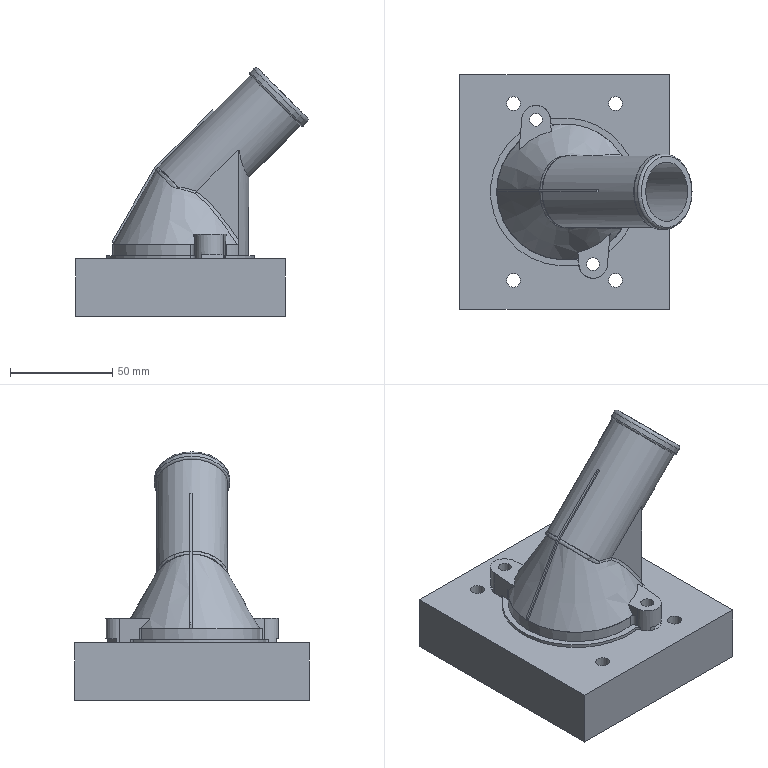NC program | NX | posted by the shop | part box 113.679 x 114.654 x 121.568 mm
Lines 15667 to 16486 of 160120:
15666 TOOL CALL 12 Z S7000
15667 CALL LBL101
15668 M3 M8
15669 M51
15670 CYCL DEF 32.0 TOLERANCE
15671 CYCL DEF 32.1 T0.012
15672 CYCL DEF 32.2 HSC-MODE:0
15673 L M126
15674 L A+0.0 C+0.0 FMAX
15675 L X31.8609 Y9.1209 FMAX
15676 L Z160.5681 FMAX
15677 L Z96.0728 FMAX
15678 L Z95.0728 F1500.
15679 CC X32.458 Y9.9231
15680 C X33.2602 Y9.326 DR+
15681 CC X46.9163 Y-.8392
15682 C X33.3788 Y9.4834 DR- F3000.
15683 CC X62.7458 Y-2.3059
15684 C X33.4604 Y9.6847 DR-
15685 L X33.5103 Y9.8057 Z95.0274
15686 L X33.5614 Y9.9262 Z94.982
15687 L X33.6113 Y10.0472 Z94.9366
15688 L X33.6604 Y10.1685 Z94.8912
15689 L X33.7117 Y10.2889 Z94.8457
15690 L X33.764 Y10.4089 Z94.8003
15691 L X33.8165 Y10.5288 Z94.7549
15692 L X33.8694 Y10.6485 Z94.7095
15693 L X33.9243 Y10.7673 Z94.6641
15694 L X33.979 Y10.8861 Z94.6187
15695 L X34.0305 Y11.0064 Z94.5732
15696 CC X54.2056 Y1.4317
15697 C X33.9017 Y10.7302 DR+
15698 CC X47.0664 Y-1.1912
15699 C X33.6839 Y10.4852 DR+
15700 L X33.7449 Y10.6101 Z94.5177
15701 L X33.8017 Y10.7386 Z94.4622
15702 L X33.8589 Y10.867 Z94.4067
15703 L X33.9187 Y10.9929 Z94.3512
15704 L X33.9813 Y11.1163 Z94.2957
15705 L X34.0439 Y11.2396 Z94.2402
15706 L X34.1065 Y11.3629 Z94.1847
15707 L X34.1699 Y11.4853 Z94.1292
15708 L X34.2302 Y11.6108 Z94.0737
15709 CC X47.4065 Y-1.7424
15710 C X34.4283 Y11.8034 DR-
15711 CC X52.6802 Y2.3208
15712 C X34.5852 Y12.0995 DR-
15713 L X34.6519 Y12.2225 Z94.0112
15714 L X34.72 Y12.3449 Z93.9488
15715 L X34.7889 Y12.4668 Z93.8863
15716 L X34.858 Y12.5886 Z93.8239
15717 L X34.9284 Y12.7096 Z93.7614
15718 L X34.9995 Y12.8303 Z93.699
15719 L X35.0713 Y12.9504 Z93.6365
15720 L X35.1434 Y13.0704 Z93.5741
15721 CC X51.7759 Y2.8978
15722 C X34.9264 Y12.7068 DR+
15723 CC X47.595 Y-2.3086
15724 C X34.6428 Y12.4629 DR+
15725 L X34.7064 Y12.5776 Z93.5027
15726 L X34.7697 Y12.6926 Z93.4314
15727 L X34.8338 Y12.8068 Z93.36
15728 L X34.898 Y12.9207 Z93.2886
15729 L X34.9625 Y13.0344 Z93.2173
15730 L X35.0272 Y13.1477 Z93.1459
15731 L X35.0935 Y13.259 Z93.0745
15732 CC X47.9658 Y-3.0564
15733 C X35.4178 Y13.5097 DR-
15734 CC X51.5003 Y3.067
15735 C X35.6579 Y13.8705 DR-
15736 L X35.7323 Y13.9762 Z93.0031
15737 L X35.8061 Y14.0823 Z92.9318
15738 L X35.8796 Y14.1887 Z92.8604
15739 L X35.9552 Y14.2937 Z92.789
15740 L X36.0312 Y14.3983 Z92.7177
15741 L X36.1073 Y14.5028 Z92.6463
15742 L X36.1847 Y14.6064 Z92.5749
15743 CC X50.2088 Y4.096
15744 C X35.9705 Y14.3144 DR+
15745 CC X35.5058 Y14.6479
15746 C X35.8306 Y14.1771 DR-
15747 CC X48.6089 Y-4.348
15748 C X35.5356 Y13.9701 DR+
15749 L X35.6164 Y14.0815 Z92.4917
15750 L X35.696 Y14.1946 Z92.4084
15751 L X35.773 Y14.3116 Z92.3252
15752 L X35.8559 Y14.42 Z92.2419
15753 L X35.9363 Y14.5319 Z92.1586
15754 L X36.0177 Y14.6424 Z92.0754
15755 CC X48.4946 Y-4.7593
15756 C X36.3569 Y14.8564 DR-
15757 CC X36.2298 Y15.0618
15758 C X36.4201 Y14.913 DR+
15759 CC X49.9995 Y4.2946
15760 C X36.6476 Y15.1977 DR-
15761 L X36.7297 Y15.297 Z91.9921
15762 L X36.8124 Y15.3958 Z91.9088
15763 L X36.8953 Y15.4945 Z91.8256
15764 L X36.9798 Y15.5918 Z91.7423
15765 L X37.065 Y15.6885 Z91.6591
15766 L X37.1494 Y15.7858 Z91.5758
15767 CC X49.6413 Y4.6277
15768 C X36.8834 Y15.4807 DR+
15769 L X36.8315 Y15.4388
15770 L X36.5049 Y15.2482
15771 CC X48.2366 Y-5.0376
15772 C X36.4144 Y15.1956 DR+
15773 L X36.4961 Y15.2878 Z91.4925
15774 L X36.5744 Y15.386 Z91.4093
15775 L X36.6545 Y15.4812 Z91.326
15776 L X36.7388 Y15.5687 Z91.2427
15777 L X36.82 Y15.6619 Z91.1595
15778 L X36.9018 Y15.7539 Z91.0762
15779 L X37.28 Y15.9541
15780 L X37.3444 Y15.9982
15781 CC X48.9822 Y5.3285
15782 C X37.6162 Y16.2873 DR-
15783 L X37.7017 Y16.3734 Z90.9763
15784 L X37.7865 Y16.4602 Z90.8764
15785 L X37.871 Y16.5474 Z90.7765
15786 L X37.9588 Y16.6311 Z90.6766
15787 L X38.0439 Y16.7177 Z90.5766
15788 CC X49.0689 Y5.1807
15789 C X37.7592 Y16.4388 DR+
15790 CC X48.7563 Y-7.1963
15791 C X37.3723 Y16.2548 DR+
15792 L X37.4643 Y16.3418 Z90.4767
15793 L X37.553 Y16.4357 Z90.3768
15794 L X37.6433 Y16.5266 Z90.2769
15795 L X37.737 Y16.6097 Z90.177
15796 L X37.8271 Y16.7009 Z90.0771
15797 CC X48.4736 Y-7.3306
15798 C X38.1814 Y16.8548 DR-
15799 L X38.2452 Y16.9038
15800 L X38.532 Y17.1609
15801 L X38.6322 Y17.2514 Z89.9522
15802 L X38.7333 Y17.3409 Z89.8273
15803 L X38.8365 Y17.428 Z89.7024
15804 L X38.9404 Y17.5143 Z89.5775
15805 CC X48.1119 Y6.4293
15806 C X38.6939 Y17.3056 DR+
15807 CC X38.3719 Y17.6775
15808 C X38.5523 Y17.2199 DR-
15809 CC X49.1499 Y-9.6613
15810 C X38.272 Y17.1077 DR+
15811 L X38.38 Y17.1938 Z89.4526
15812 L X38.4867 Y17.2833 Z89.3277
15813 L X38.5921 Y17.3758 Z89.2028
15814 L X38.6977 Y17.4684 Z89.0779
15815 CC X49.149 Y-10.7005
15816 C X39.0373 Y17.5921 DR-
15817 CC X48.0093 Y6.6011
15818 C X39.2967 Y17.7988 DR-
15819 L X39.3977 Y17.8756 Z88.953
15820 L X39.4982 Y17.9531 Z88.8281
15821 L X39.6008 Y18.0278 Z88.7032
15822 L X39.7031 Y18.1029 Z88.5783
15823 CC X47.8447 Y6.8745
15824 C X39.5096 Y17.9601 DR+
15825 CC X39.045 Y18.5781
15826 C X39.2845 Y17.8429 DR-
15827 CC X48.4793 Y-10.3807
15828 C X39.0206 Y17.7556 DR+
15829 L X39.1137 Y17.8261 Z88.4534
15830 L X39.2068 Y17.8968 Z88.3286
15831 L X39.301 Y17.9637 Z88.2037
15832 L X39.3929 Y18.0383 Z88.0788
15833 CC X48.1341 Y-10.6842
15834 C X39.7332 Y18.1397 DR-
15835 L X39.8002 Y18.1734
15836 L X39.9416 Y18.2715
15837 CC X47.5875 Y7.3222
15838 C X40.0707 Y18.3605 DR-
15839 L X40.1695 Y18.4271 Z87.9539
15840 L X40.2694 Y18.4921 Z87.829
15841 L X40.3693 Y18.5571 Z87.7041
15842 L X40.472 Y18.6176 Z87.5792
15843 L X40.1807 Y18.4348
15844 L X40.0829 Y18.3797
15845 CC X48.0743 Y-11.786
15846 C X39.7228 Y18.282 DR+
15847 L X39.8204 Y18.3515 Z87.4127
15848 L X39.9172 Y18.4238 Z87.2461
15849 L X40.0148 Y18.4934 Z87.0796
15850 CC X47.5569 Y-11.6861
15851 C X40.0829 Y18.5104 DR-
15852 L X40.3657 Y18.5825
15853 CC X40.2689 Y18.99
15854 C X40.507 Y18.6454 DR+
15855 L X40.7256 Y18.7769
15856 L X40.8118 Y18.8292 Z86.9131
15857 L X40.8988 Y18.8803 Z86.7466
15858 L X40.9852 Y18.9324 Z86.58
15859 CC X47.4204 Y7.6609
15860 C X40.7217 Y18.7778 DR+
15861 CC X48.263 Y-15.7413
15862 C X40.3289 Y18.6897 DR+
15863 L X40.4108 Y18.7449 Z86.4135
15864 L X40.4934 Y18.7971 Z86.247
15865 L X40.5754 Y18.8516 Z86.0805
15866 CC X47.5853 Y-15.1069
15867 C X40.9311 Y18.9231 DR-
15868 L X41.0725 Y18.9785
15869 L X41.2139 Y19.0569
15870 CC X47.2578 Y8.1038
15871 C X41.2978 Y19.1027 DR-
15872 L X41.3989 Y19.1555 Z85.9139
15873 L X41.5002 Y19.2079 Z85.7474
15874 L X41.6018 Y19.2595 Z85.5809
15875 L X41.276 Y19.0932
15876 CC X41.1349 Y19.3697
15877 C X41.2139 Y19.0694 DR-
15878 CC X47.3266 Y-16.0557
15879 C X40.8867 Y19.0109 DR+
15880 L X40.9673 Y19.0682 Z85.3311
15881 L X41.0484 Y19.1231 Z85.0813
15882 CC X46.4514 Y-14.5078
15883 C X41.4282 Y19.1819 DR-
15884 CC X41.4031 Y19.35
15885 C X41.48 Y19.1984 DR+
15886 L X41.6401 Y19.2797
15887 CC X47.2127 Y8.2615
15888 C X41.7839 Y19.3513 DR-
15889 L X41.8645 Y19.3891 Z84.8315
15890 L X41.9434 Y19.4305 Z84.5817
15891 CC X47.5312 Y7.3302
15892 C X41.6385 Y19.2849 DR+
15893 CC X46.1296 Y-15.1859
15894 C X41.239 Y19.2305 DR+
15895 L X41.3086 Y19.2709 Z84.3319
15896 L X41.3779 Y19.3138 Z84.0822
15897 CC X45.6127 Y-15.1548
15898 C X41.7793 Y19.3608 DR-
15899 L X41.8553 Y19.3856
15900 L X42.1605 Y19.5244
15901 L X42.2293 Y19.5564 Z83.8324
15902 L X42.2988 Y19.5867 Z83.5826
15903 CC X47.2002 Y8.3445
15904 C X42.2611 Y19.5702 DR+
15905 L X41.9951 Y19.4518
15906 L X41.926 Y19.4302
15907 CC X45.2379 Y-15.7261
15908 C X41.5806 Y19.3959 DR+
15909 L X41.6218 Y19.4479 Z83.083
15910 CC X44.6983 Y-15.5102
15911 C X42.0621 Y19.4839 DR-
15912 CC X47.212 Y8.2577
15913 C X42.4025 Y19.6339 DR-
15914 L X42.4899 Y19.6685 Z82.5834
15915 CC X47.2024 Y8.3283
15916 C X42.1632 Y19.5272 DR+
15917 CC X44.2618 Y-15.76
15918 C X41.7612 Y19.501 DR+
15919 L X41.6982 Y19.5286 Z82.0839
15920 CC X43.7723 Y-15.8546
15921 C X42.2265 Y19.5556 DR-
15922 CC X47.2028 Y8.3242
15923 C X42.6208 Y19.7222 DR-
15924 L X42.6468 Y19.7357 Z81.5843
15925 CC X47.2378 Y8.1081
15926 C X42.2601 Y19.5755 DR+
15927 CC X43.2847 Y-15.9241
15928 C X41.7551 Y19.5573 DR+
15929 L X41.7635 Y19.5754 Z81.0847
15930 CC X42.7728 Y-15.8382
15931 C X42.258 Y19.586 DR-
15932 L X42.3281 Y19.5996
15933 L X42.6275 Y19.7228
15934 CC X47.1919 Y8.4075
15935 C X42.7343 Y19.7652 DR-
15936 L X42.7859 Y19.7874 Z80.5851
15937 CC X47.2035 Y8.3175
15938 C X42.3229 Y19.5982 DR+
15939 CC X42.3953 Y-16.4936
15940 C X41.7352 Y19.5922 DR+
15941 L X41.7262 Y19.5999 Z80.0856
15942 CC X42.0068 Y-17.6204
15943 C X42.3281 Y19.5996 DR-
15944 CC X47.2003 Y8.3424
15945 C X42.791 Y19.7888 DR-
15946 L Z79.586
15947 CC X47.2003 Y8.3424
15948 C X42.3281 Y19.5996 DR+
15949 CC X41.9084 Y-33.373
15950 C X41.7097 Y19.6009 DR+
15951 L X41.6899 Y19.5996 Z79.0864
15952 L X42.3281
15953 CC X47.2003 Y8.3424
15954 C X42.7932 Y19.7897 DR-
15955 L Z78.5868
15956 CC X47.2003 Y8.3424
15957 C X42.3281 Y19.5996 DR+
15958 CC X41.4246 Y-60.9014
15959 C X41.7442 Y19.604 DR+
15960 L X41.7538 Y19.6049 Z78.0873
15961 CC X41.1736 Y-74.9474
15962 C X42.3281 Y19.5996 DR-
15963 CC X47.2003 Y8.3424
15964 C X42.7932 Y19.7897 DR-
15965 L Z77.5877
15966 CC X47.2003 Y8.3424
15967 C X42.3281 Y19.5996 DR+
15968 CC X40.9092 Y-86.8141
15969 C X41.7624 Y19.6056 DR+
15970 L X41.6906 Y19.5996 Z77.0881
15971 L X42.3281
15972 CC X47.2003 Y8.3424
15973 C X42.7932 Y19.7897 DR-
15974 L Z76.5885
15975 CC X47.2002 Y8.3424
15976 C X42.3281 Y19.5996 DR+
15977 CC X40.4559 Y-118.8545
15978 C X41.767 Y19.6061 DR+
15979 L X41.7725 Y19.6066 Z76.089
15980 CC X40.1882 Y-129.1976
15981 C X42.3281 Y19.5996 DR-
15982 CC X47.2002 Y8.3424
15983 C X42.7932 Y19.7897 DR-
15984 L Z75.5894
15985 CC X47.2002 Y8.3425
15986 C X42.3281 Y19.5996 DR+
15987 L X41.691 Y19.5997
15988 L X41.6909 Z75.0898
15989 L X42.3281 Y19.5996
15990 CC X47.2002 Y8.3425
15991 C X42.7932 Y19.7897 DR-
15992 L Z74.5902
15993 CC X47.2002 Y8.3425
15994 C X42.3281 Y19.5996 DR+
15995 L X41.6899
15996 L X41.6908 Y19.5997 Z74.0907
15997 L X42.3281 Y19.5996
15998 CC X47.2002 Y8.3425
15999 C X42.7932 Y19.7897 DR-
16000 L Z73.5911
16001 CC X47.2002 Y8.3425
16002 C X42.3281 Y19.5996 DR+
16003 L X41.6908 Y19.5997
16004 L X41.6907 Z73.0915
16005 L X42.3281 Y19.5996
16006 CC X47.2002 Y8.3425
16007 C X42.7932 Y19.7897 DR-
16008 L Z72.5919
16009 CC X47.2002 Y8.3425
16010 C X42.3281 Y19.5996 DR+
16011 L X41.6901
16012 L X41.6907 Y19.5997 Z72.0924
16013 L X42.3281 Y19.5996
16014 CC X47.2002 Y8.3425
16015 C X42.7932 Y19.7897 DR-
16016 L Z71.5928
16017 CC X47.2002 Y8.3425
16018 C X42.3281 Y19.5997 DR+
16019 L X41.6907
16020 L X41.6906 Z71.0932
16021 L X42.3281
16022 CC X47.2002 Y8.3425
16023 C X42.7932 Y19.7897 DR-
16024 L Z70.5936
16025 CC X47.2001 Y8.3425
16026 C X42.3281 Y19.5997 DR+
16027 L X41.6906
16028 L X41.6908 Z70.0941
16029 L X42.3281
16030 CC X47.2001 Y8.3425
16031 C X42.7932 Y19.7898 DR-
16032 L Z69.5945
16033 CC X47.2001 Y8.3425
16034 C X42.3281 Y19.5997 DR+
16035 L X41.6908
16036 L Z69.0949
16037 L X42.3281
16038 CC X47.2001 Y8.3425
16039 C X42.7932 Y19.7898 DR-
16040 L Z68.5953
16041 CC X47.2001 Y8.3425
16042 C X42.3281 Y19.5997 DR+
16043 L X41.6906
16044 L X41.6901 Z68.0958
16045 L X42.3281
16046 CC X47.2001 Y8.3425
16047 C X42.7932 Y19.7898 DR-
16048 L Z67.5962
16049 CC X47.2001 Y8.3426
16050 C X42.3281 Y19.5997 DR+
16051 L X41.6904
16052 L X41.6907 Z67.0966
16053 L X42.3281
16054 CC X47.2001 Y8.3426
16055 C X42.7932 Y19.7898 DR-
16056 L Z66.597
16057 CC X47.2001 Y8.3426
16058 C X42.3281 Y19.5997 DR+
16059 L X41.6907
16060 L X41.6903 Z66.0975
16061 L X42.3281
16062 CC X47.2001 Y8.3426
16063 C X42.7932 Y19.7898 DR-
16064 L Z65.5979
16065 CC X47.2001 Y8.3426
16066 C X42.3281 Y19.5997 DR+
16067 L X41.6906
16068 L X41.6936 Y19.6 Z65.0983
16069 L X42.3281 Y19.5997
16070 CC X47.2001 Y8.3426
16071 C X42.7932 Y19.7898 DR-
16072 CC X42.434 Y20.723
16073 C X43.3672 Y21.0823 DR+
16074 L Z66.0983
16075 L Z160.5681 FMAX
16076 L X33.5558 Y-12.3385 FMAX
16077 L Z95.5732 FMAX
16078 L Z94.5732 F1500.
16079 CC X33.1271 Y-11.4351
16080 C X34.0305 Y-11.0064 DR+
16081 CC X54.2036 Y-1.4327
16082 C X33.9017 Y-10.7302 DR- F3000.
16083 CC X47.0951 Y1.2135
16084 C X33.6837 Y-10.4848 DR-
16085 L X33.7446 Y-10.6097 Z94.5177
16086 L X33.8015 Y-10.7383 Z94.4622
16087 L X33.8587 Y-10.8667 Z94.4067
16088 L X33.9186 Y-10.9927 Z94.3512
16089 L X33.9812 Y-11.1161 Z94.2957
16090 L X34.0438 Y-11.2395 Z94.2402
16091 L X34.1064 Y-11.3628 Z94.1847
16092 L X34.1699 Y-11.4852 Z94.1292
16093 L X34.2302 Y-11.6108 Z94.0737
16094 CC X47.4065 Y1.7424
16095 C X34.4283 Y-11.8034 DR+
16096 CC X52.6939 Y-2.313
16097 C X34.5852 Y-12.0996 DR+
16098 L X34.6519 Y-12.2227 Z94.0112
16099 L X34.7199 Y-12.345 Z93.9488
16100 L X34.7888 Y-12.4669 Z93.8863
16101 L X34.858 Y-12.5887 Z93.8239
16102 L X34.9284 Y-12.7097 Z93.7614
16103 L X34.9995 Y-12.8303 Z93.699
16104 L X35.0713 Y-12.9504 Z93.6365
16105 L X35.1434 Y-13.0704 Z93.5741
16106 CC X51.7755 Y-2.898
16107 C X34.9264 Y-12.7068 DR-
16108 CC X47.4839 Y2.1983
16109 C X34.6444 Y-12.4646 DR-
16110 L X34.7091 Y-12.5799 Z93.5027
16111 L X34.7734 Y-12.6957 Z93.4314
16112 L X34.8384 Y-12.8107 Z93.36
16113 L X34.9037 Y-12.9254 Z93.2886
16114 L X34.9691 Y-13.0399 Z93.2173
16115 L X35.0348 Y-13.1541 Z93.1459
16116 L X35.1017 Y-13.2668 Z93.0745
16117 CC X47.8102 Y2.9421
16118 C X35.4178 Y-13.5097 DR+
16119 CC X51.4895 Y-3.0751
16120 C X35.6578 Y-13.8703 DR+
16121 L X35.7329 Y-13.976 Z93.0031
16122 L X35.806 Y-14.0831 Z92.9318
16123 L X35.8799 Y-14.1896 Z92.8604
16124 L X35.956 Y-14.2946 Z92.789
16125 L X36.0322 Y-14.3995 Z92.7177
16126 L X36.1085 Y-14.5044 Z92.6463
16127 L X36.1862 Y-14.6081 Z92.5749
16128 CC X50.4874 Y-3.8763
16129 C X35.9314 Y-14.2599 DR-
16130 L X35.8419 Y-14.1849
16131 L X35.5229 Y-13.9593
16132 L X35.6051 Y-14.0736 Z92.4917
16133 L X35.6871 Y-14.1882 Z92.4084
16134 L X35.7662 Y-14.307 Z92.3252
16135 L X35.8515 Y-14.4168 Z92.2419
16136 L X35.9342 Y-14.5304 Z92.1586
16137 L X36.0179 Y-14.6425 Z92.0754
16138 CC X48.466 Y4.7153
16139 C X36.3544 Y-14.8548 DR+
16140 CC X36.2184 Y-15.0745
16141 C X36.4219 Y-14.9153 DR-
16142 CC X49.9984 Y-4.2957
16143 C X36.6476 Y-15.1977 DR+
16144 L X36.7295 Y-15.2974 Z91.9921
16145 L X36.8126 Y-15.396 Z91.9088
16146 L X36.8956 Y-15.4949 Z91.8256
16147 L X36.9802 Y-15.5923 Z91.7423
16148 L X37.0655 Y-15.6891 Z91.6591
16149 L X37.15 Y-15.7865 Z91.5758
16150 CC X49.6268 Y-4.6419
16151 C X36.8834 Y-15.4807 DR-
16152 L X36.8315 Y-15.4388
16153 L X36.5049 Y-15.2482
16154 CC X48.2366 Y5.0376
16155 C X36.4144 Y-15.1956 DR-
16156 L X36.4961 Y-15.2878 Z91.4925
16157 L X36.5745 Y-15.386 Z91.4093
16158 L X36.6546 Y-15.4812 Z91.326
16159 L X36.7389 Y-15.5688 Z91.2427
16160 L X36.8201 Y-15.662 Z91.1595
16161 L X36.9019 Y-15.754 Z91.0762
16162 L X37.28 Y-15.9541
16163 L X37.3444 Y-15.9982
16164 CC X48.9668 Y-5.3455
16165 C X37.6133 Y-16.2844 DR+
16166 L X37.699 Y-16.3714 Z90.9763
16167 L X37.7847 Y-16.4585 Z90.8764
16168 L X37.8697 Y-16.5462 Z90.7765
16169 L X37.9582 Y-16.6305 Z90.6766
16170 L X38.0438 Y-16.7176 Z90.5766
16171 CC X49.0657 Y-5.1845
16172 C X37.7592 Y-16.4388 DR-
16173 CC X48.6548 Y7.0045
16174 C X37.3737 Y-16.2557 DR-
16175 L X37.4657 Y-16.3425 Z90.4767
16176 L X37.5544 Y-16.4364 Z90.3768
16177 L X37.6445 Y-16.5272 Z90.2769
16178 L X37.7382 Y-16.6102 Z90.177
16179 L X37.8281 Y-16.7015 Z90.0771
16180 CC X48.8219 Y8.1511
16181 C X38.1814 Y-16.8548 DR+
16182 L X38.2452 Y-16.9038
16183 CC X48.3508 Y-6.0948
16184 C X38.5023 Y-17.1385 DR+
16185 L X38.5887 Y-17.2154 Z89.9772
16186 L X38.6761 Y-17.2912 Z89.8772
16187 L X38.7637 Y-17.3668 Z89.7773
16188 L X38.8522 Y-17.4414 Z89.6774
16189 L X38.9414 Y-17.515 Z89.5775
16190 CC X48.1565 Y-6.3691
16191 C X38.6693 Y-17.2843 DR-
16192 L X38.5756 Y-17.2248
16193 CC X48.8901 Y9.2101
16194 C X38.2438 Y-17.0929 DR-
16195 L X38.3359 Y-17.1647 Z89.4776
16196 L X38.426 Y-17.2414 Z89.3777
16197 L X38.5178 Y-17.3139 Z89.2777
16198 L X38.6076 Y-17.3914 Z89.1778
16199 L X38.6977 Y-17.4684 Z89.0779
16200 CC X49.149 Y10.7006
16201 C X39.0373 Y-17.5921 DR+
16202 CC X48.005 Y-6.6065
16203 C X39.2967 Y-17.7988 DR+
16204 L X39.397 Y-17.8766 Z88.953
16205 L X39.4985 Y-17.9528 Z88.8281
16206 L X39.601 Y-18.0277 Z88.7032
16207 L X39.7034 Y-18.1027 Z88.5783
16208 CC X47.7129 Y-7.0909
16209 C X39.5068 Y-17.957 DR-
16210 CC X39.0694 Y-18.5361
16211 C X39.294 Y-17.846 DR+
16212 CC X48.4793 Y10.3807
16213 C X39.0206 Y-17.7556 DR-
16214 L X39.1137 Y-17.8261 Z88.4534
16215 L X39.2068 Y-17.8968 Z88.3286
16216 L X39.301 Y-17.9637 Z88.2037
16217 L X39.3929 Y-18.0383 Z88.0788
16218 CC X48.1341 Y10.6842
16219 C X39.7332 Y-18.1397 DR+
16220 L X39.8002 Y-18.1734
16221 L X39.9416 Y-18.2715
16222 CC X47.5925 Y-7.312
16223 C X40.0709 Y-18.3606 DR+
16224 L X40.1609 Y-18.4216 Z87.9539
16225 L X40.2521 Y-18.4808 Z87.829
16226 L X40.3431 Y-18.5402 Z87.7041
16227 L X40.4348 Y-18.5986 Z87.5792
16228 L X40.1807 Y-18.4348
16229 L X40.0829 Y-18.3797
16230 CC X48.0743 Y11.786
16231 C X39.7228 Y-18.282 DR-
16232 L X39.8203 Y-18.3515 Z87.4127
16233 L X39.9172 Y-18.4238 Z87.2461
16234 L X40.0147 Y-18.4934 Z87.0796
16235 CC X47.5569 Y11.6861
16236 C X40.0829 Y-18.5104 DR+
16237 L X40.3657 Y-18.5825
16238 CC X40.2689 Y-18.99
16239 C X40.507 Y-18.6454 DR-
16240 L X40.7257 Y-18.777
16241 L X40.8128 Y-18.8297 Z86.9131
16242 L X40.9006 Y-18.8811 Z86.7466
16243 L X40.9878 Y-18.9335 Z86.58
16244 CC X47.4806 Y-7.5327
16245 C X40.7217 Y-18.7778 DR-
16246 CC X48.0343 Y14.8569
16247 C X40.3336 Y-18.6911 DR-
16248 L X40.414 Y-18.7455 Z86.4135
16249 L X40.495 Y-18.7974 Z86.247
16250 L X40.5755 Y-18.8517 Z86.0805
16251 CC X47.5584 Y14.9783
16252 C X40.9126 Y-18.9195 DR+
16253 CC X40.822 Y-19.3818
16254 C X41.0437 Y-18.9661 DR-
16255 L X41.3059 Y-19.1061
16256 L X41.4005 Y-19.1562 Z85.9139
16257 L X41.4951 Y-19.2064 Z85.7474
16258 L X41.5907 Y-19.2546 Z85.5809
16259 CC X47.1817 Y-8.3438
16260 C X41.4879 Y-19.2014 DR-
16261 L X41.2862 Y-19.0955
16262 L X41.2139 Y-19.0695
16263 CC X47.3277 Y16.0599
16264 C X40.8868 Y-19.011 DR-
16265 L X40.9611 Y-19.0669 Z85.3311
16266 L X41.0359 Y-19.1199 Z85.0813
16267 L X41.2139 Y-19.148
16268 L X41.4547 Y-19.1902
16269 CC X41.4352 Y-19.302
16270 C X41.4878 Y-19.2014 DR-
16271 CC X47.2065 Y-8.2714
16272 C X41.7839 Y-19.3513 DR+
16273 L X41.8762 Y-19.3948 Z84.8315
16274 L X41.9682 Y-19.4392 Z84.5817
16275 CC X47.208 Y-8.2835
16276 C X41.8554 Y-19.3855 DR-
16277 L X41.7684 Y-19.3426
16278 L X41.6384 Y-19.2851
16279 CC X46.1358 Y15.2083
16280 C X41.2388 Y-19.2307 DR-
16281 L X41.301 Y-19.2697 Z84.3319
16282 L X41.363 Y-19.3101 Z84.0822
16283 CC X45.6083 Y15.1726
16284 C X41.7459 Y-19.3551 DR+
16285 CC X41.715 Y-19.6314
16286 C X41.8281 Y-19.3774 DR-
16287 L X42.0621 Y-19.4815
16288 CC X47.2016 Y-8.3236
16289 C X42.1562 Y-19.5244 DR+
16290 L X42.228 Y-19.556 Z83.8324
16291 L X42.2999 Y-19.5874 Z83.5826
16292 CC X47.1975 Y-8.3492
16293 C X42.1936 Y-19.5404 DR-
16294 CC X40.1986 Y-24.002
16295 C X41.926 Y-19.4302 DR+
16296 CC X45.1816 Y15.389
16297 C X41.5804 Y-19.3961 DR-
16298 L X41.6247 Y-19.4481 Z83.083
16299 CC X44.7081 Y15.5594
16300 C X42.0621 Y-19.4839 DR+
16301 CC X47.2117 Y-8.2562
16302 C X42.4272 Y-19.6443 DR+
16303 L X42.5361 Y-19.6876 Z82.5834
16304 CC X47.1997 Y-8.336
16305 C X42.1633 Y-19.5272 DR-
16306 CC X44.2675 Y15.789
16307 C X41.6956 Y-19.4962 DR-
16308 L X41.6979 Y-19.5151 Z82.3336
16309 L X41.6995 Y-19.5289 Z82.0839
16310 CC X43.7807 Y15.897
16311 C X42.2283 Y-19.556 DR+
16312 CC X47.1975 Y-8.3486
16313 C X42.6217 Y-19.7222 DR+
16314 L X42.6453 Y-19.7351 Z81.5843
16315 CC X47.2574 Y-8.0517
16316 C X42.26 Y-19.5756 DR-
16317 L X42.2333 Y-19.58
16318 L X41.7234 Y-19.5532
16319 L X41.7628 Y-19.5749 Z81.0847
16320 CC X42.7699 Y15.831
16321 C X42.0621 Y-19.5822 DR+
16322 L X42.2732 Y-19.5875
16323 CC X42.2694 Y-19.7351
16324 C X42.3281 Y-19.5996 DR-
16325 CC X47.1963 Y-8.3549
16326 C X42.7162 Y-19.7598 DR+
16327 L X42.7856 Y-19.7873 Z80.5851
16328 CC X47.2005 Y-8.326
16329 C X42.3229 Y-19.5982 DR-
16330 CC X42.3894 Y16.4551
16331 C X41.7346 Y-19.5923 DR-
16332 L X41.7323 Y-19.6006 Z80.0856
16333 CC X41.9681 Y17.0175
16334 C X42.3281 Y-19.5996 DR+
16335 CC X47.1963 Y-8.3548
16336 C X42.7904 Y-19.7886 DR+
16337 L Y-19.7887 Z79.586
16338 CC X47.1963 Y-8.3548
16339 C X42.3281 Y-19.5996 DR-
16340 CC X41.7486 Y22.1907
16341 C X41.7425 Y-19.6036 DR-
16342 L X41.7431 Y-19.6039 Z79.0864
16343 CC X41.6147 Y37.4775
16344 C X42.3281 Y-19.5996 DR+
16345 CC X47.1963 Y-8.3549
16346 C X42.7927 Y-19.7895 DR+
16347 L Z78.5868
16348 CC X47.1963 Y-8.3549
16349 C X42.3281 Y-19.5996 DR-
16350 CC X41.5139 Y73.0102
16351 C X41.7315 Y-19.6029 DR-
16352 L X41.7531 Y-19.6048 Z78.0873
16353 CC X41.1758 Y76.0799
16354 C X42.3281 Y-19.5996 DR+
16355 CC X47.1963 Y-8.3549
16356 C X42.7927 Y-19.7895 DR+
16357 L Z77.5877
16358 CC X47.1963 Y-8.3549
16359 C X42.3281 Y-19.5996 DR-
16360 CC X40.9146 Y88.3829
16361 C X41.7614 Y-19.6055 DR-
16362 L X41.7805 Y-19.6073 Z77.0881
16363 CC X40.6364 Y81.5855
16364 C X42.3281 Y-19.5996 DR+
16365 CC X47.1963 Y-8.3549
16366 C X42.7927 Y-19.7895 DR+
16367 L Z76.5885
16368 CC X47.1962 Y-8.3549
16369 C X42.3281 Y-19.5996 DR-
16370 L X41.6843 Y-19.5991
16371 L X41.7706 Y-19.6064 Z76.089
16372 CC X40.1974 Y132.9569
16373 C X42.3281 Y-19.5996 DR+
16374 CC X47.1962 Y-8.3549
16375 C X42.7927 Y-19.7895 DR+
16376 L Y-19.7896 Z75.5894
16377 CC X47.1962 Y-8.355
16378 C X42.3281 Y-19.5996 DR-
16379 L X41.6873 Y-19.5994
16380 L X41.6953 Y-19.6 Z75.0898
16381 L X42.3281 Y-19.5996
16382 CC X47.1962 Y-8.355
16383 C X42.7927 Y-19.7896 DR+
16384 L Z74.5902
16385 CC X47.1962 Y-8.355
16386 C X42.3281 Y-19.5996 DR-
16387 L X41.6945 Y-19.6
16388 L X41.69 Y-19.5996 Z74.0907
16389 L X42.3281
16390 CC X47.1962 Y-8.355
16391 C X42.7927 Y-19.7896 DR+
16392 L Z73.5911
16393 CC X47.1962 Y-8.355
16394 C X42.3281 Y-19.5997 DR-
16395 L X41.691
16396 L Z73.0915
16397 L X42.3281
16398 CC X47.1961 Y-8.355
16399 C X42.7927 Y-19.7896 DR+
16400 L Z72.5919
16401 CC X47.1961 Y-8.355
16402 C X42.3281 Y-19.5997 DR-
16403 L X41.6946 Y-19.6
16404 L X41.6902 Y-19.5996 Z72.0924
16405 L X42.3281 Y-19.5997
16406 CC X47.1961 Y-8.3551
16407 C X42.7927 Y-19.7896 DR+
16408 L Z71.5928
16409 CC X47.1961 Y-8.3551
16410 C X42.3281 Y-19.5997 DR-
16411 L X41.6896 Y-19.5996
16412 L X41.6909 Y-19.5997 Z71.0932
16413 L X42.3281
16414 CC X47.1961 Y-8.3551
16415 C X42.7927 Y-19.7896 DR+
16416 L Z70.5936
16417 CC X47.1961 Y-8.3551
16418 C X42.3281 Y-19.5997 DR-
16419 L X41.6908
16420 L X41.6906 Z70.0941
16421 L X42.3281
16422 CC X47.1961 Y-8.3551
16423 C X42.7927 Y-19.7896 DR+
16424 L Z69.5945
16425 CC X47.1961 Y-8.3551
16426 C X42.3281 Y-19.5997 DR-
16427 L X41.691
16428 L Z69.0949
16429 L X42.3281
16430 CC X47.196 Y-8.3552
16431 C X42.7927 Y-19.7896 DR+
16432 L Z68.5953
16433 CC X47.196 Y-8.3552
16434 C X42.3281 Y-19.5997 DR-
16435 L X41.6908
16436 L X41.6904 Z68.0958
16437 L X42.3281
16438 CC X47.196 Y-8.3552
16439 C X42.7927 Y-19.7896 DR+
16440 L Z67.5962
16441 CC X47.196 Y-8.3552
16442 C X42.3281 Y-19.5997 DR-
16443 L X41.6906
16444 L X41.6907 Z67.0966
16445 L X42.3281
16446 CC X47.196 Y-8.3552
16447 C X42.7927 Y-19.7896 DR+
16448 L Z66.597
16449 CC X47.196 Y-8.3552
16450 C X42.3281 Y-19.5997 DR-
16451 L X41.6909
16452 L X41.6905 Z66.0975
16453 L X42.3281
16454 CC X47.196 Y-8.3552
16455 C X42.7927 Y-19.7896 DR+
16456 L Z65.5979
16457 CC X47.1959 Y-8.3553
16458 C X42.3281 Y-19.5997 DR-
16459 L X41.6905
16460 L X41.6936 Y-19.6 Z65.0983
16461 L X42.3281 Y-19.5997
16462 CC X47.1959 Y-8.3553
16463 C X42.7927 Y-19.7897 DR+
16464 CC X42.4333 Y-20.7228
16465 C X43.3665 Y-21.0822 DR-
16466 L Z66.0983
16467 L Z92.5758 FMAX
16468 L X13.1056 Y2.9957 F10000.
16469 L Z81.0856 FMAX
16470 L Z80.0856 F1500.
16471 CC X13.9332 Y3.5571
16472 C X14.4946 Y2.7296 DR+
16473 CC X15.6747 Y.99
16474 C X15.3889 Y3.0726 DR- F3000.
16475 CC X31.1286 Y-.4108
16476 C X15.8238 Y4.6523 DR-
16477 L X15.6971 Y4.6541 Z79.9607
16478 L X15.572 Y4.6553 Z79.8358
16479 L X15.4469 Y4.6565 Z79.7109
16480 L X15.3257 Y4.6564 Z79.586
16481 CC X30.6269 Y-.4095
16482 C X14.8902 Y3.0759 DR+
16483 CC X15.1834 Y.9852
16484 C X13.9811 Y2.7205 DR+
16485 L X13.8583 Y2.7171 Z79.4611